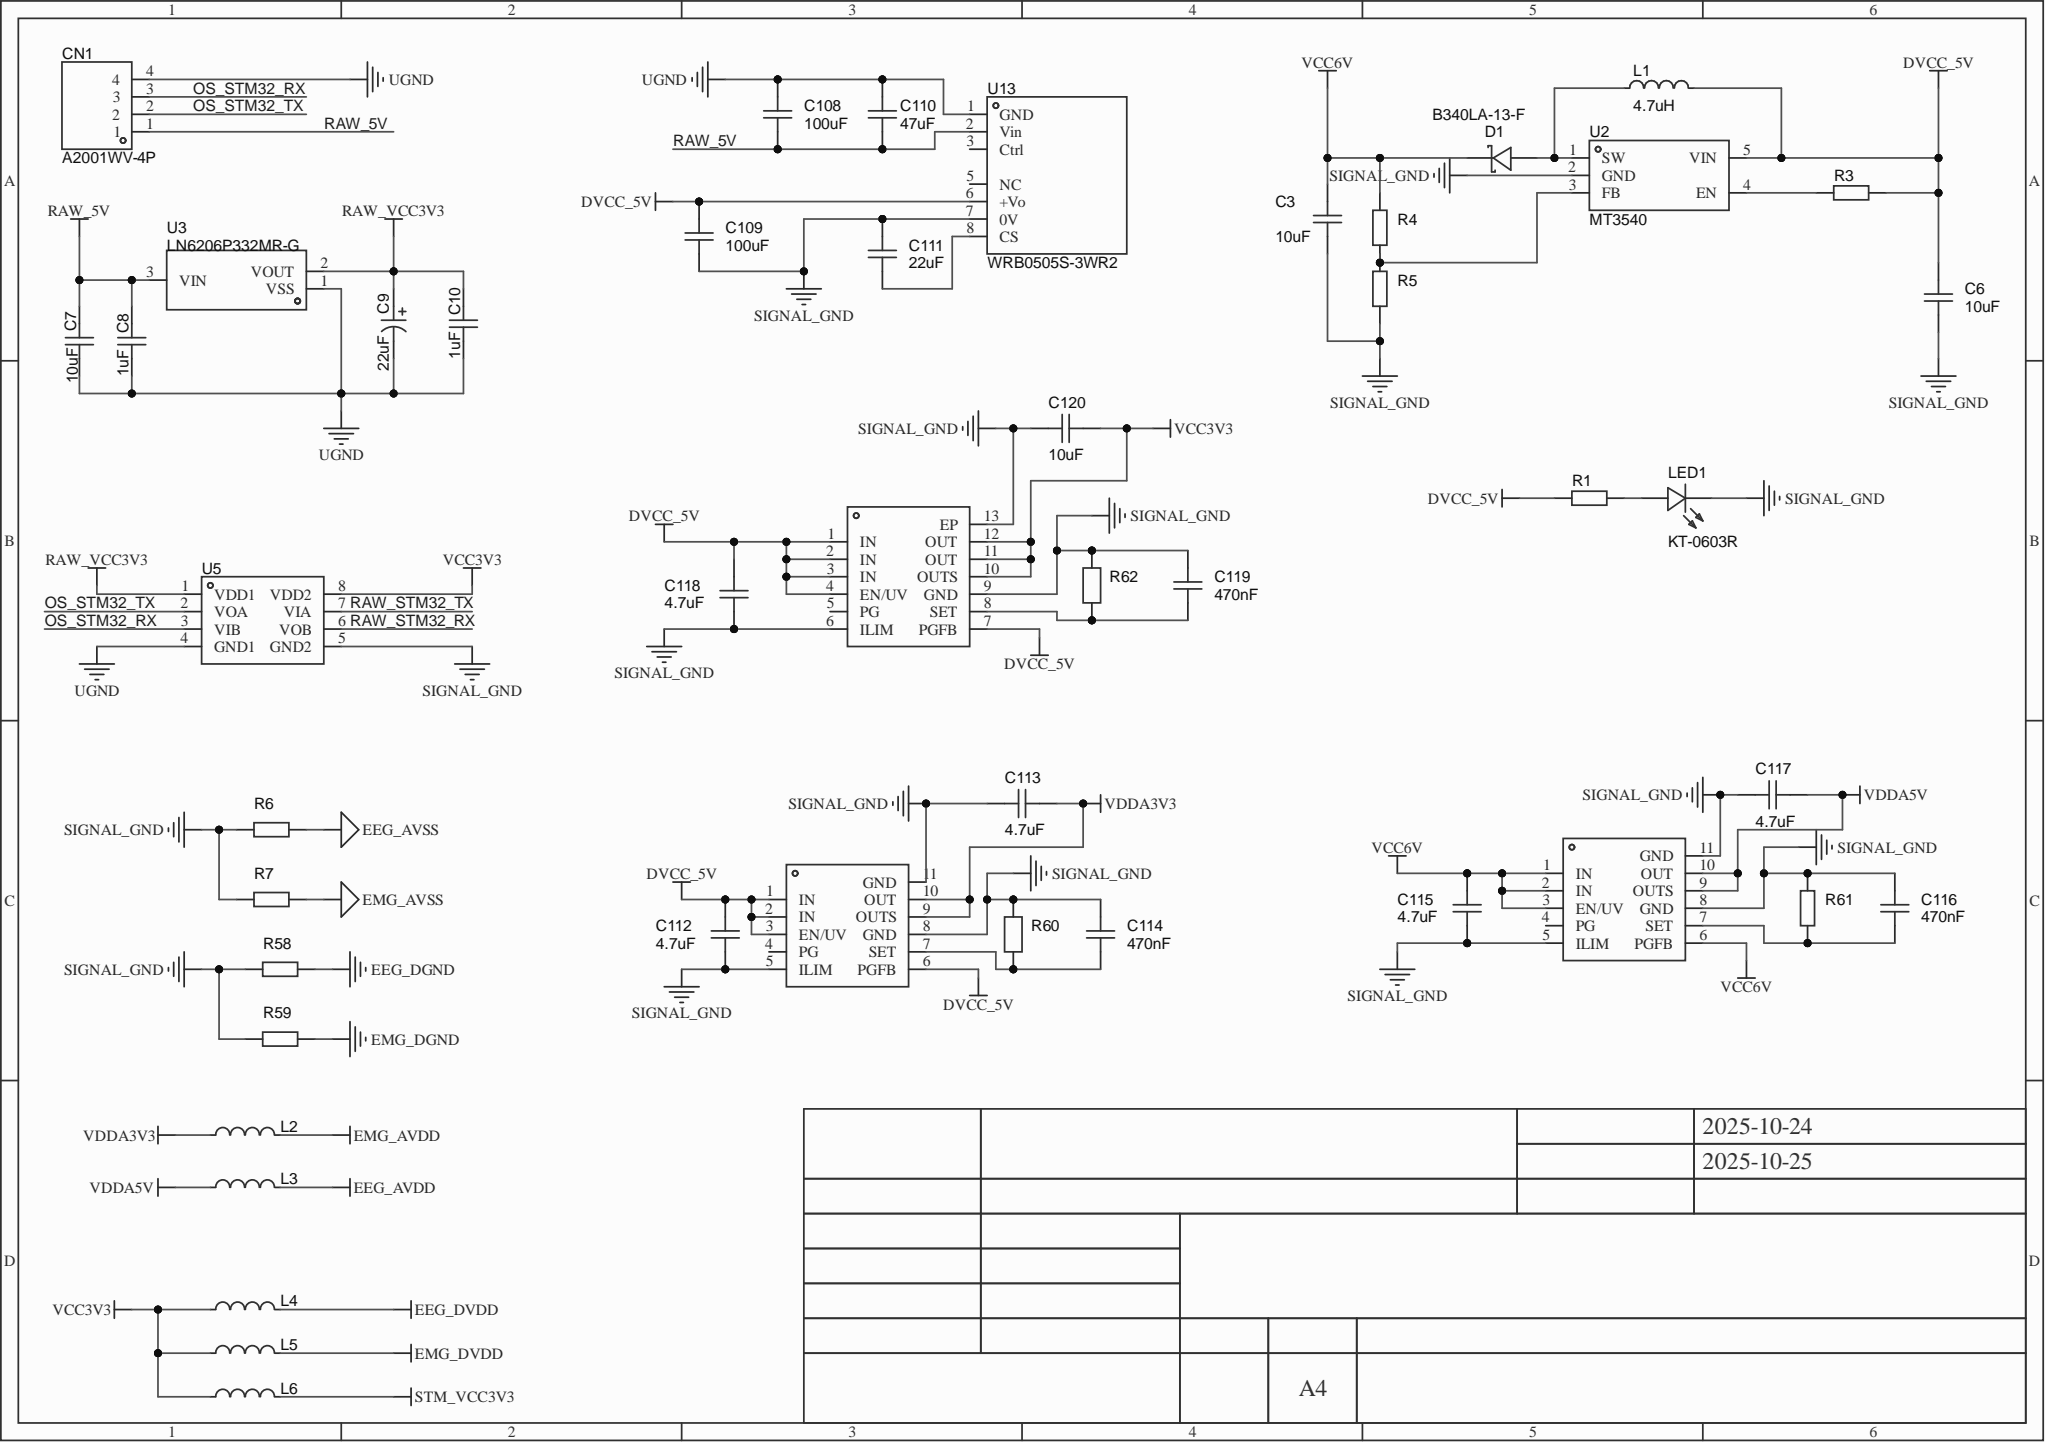Circuit board | Altium Designer | 211 parts | 126 nets | one sheet of the schematic
Parts on this sheet (reference | value | footprint):
C3 | 10uF | C0603
C6 | 10uF | C0603
C7 | 10uF | C0603
C8 | 1uF | C0402
C9 | 22uF | CAP-SMD_L3.2-W1.6
C10 | 1uF | C0402
C108 | 100uF | C1206
C109 | 100uF | C1206
C110 | 47uF | C1206
C111 | 22uF | C1206
C112 | 4.7uF | C0603
C113 | 4.7uF | C0603
C114 | 470nF | C0603
C115 | 4.7uF | C0603
C116 | 470nF | C0603
C117 | 4.7uF | C0603
C118 | 4.7uF | C0603
C119 | 470nF | C0603
C120 | 10uF | C0603
CN1 | A2001WV-4P | CONN-TH_A2001WV-4P
D1 | B340LA-13-F | SMA_L4.3-W2.6-LS5.2-RD
L1 | 4.7uH | IND-SMD_L4.0-W4.0_FNR40XXS
L2 | BLM15PD121SN1D | L0402
L3 | BLM15PD121SN1D | L0402
L4 | BLM15PD121SN1D | L0402
L5 | BLM15PD121SN1D | L0402
L6 | BLM15PD121SN1D | L0402
LED1 | KT-0603R | LED0603-RD
R1 | R0603
R3 | R0402
R4 | R0402
R5 | R0402
R6 | R0402
R7 | R0402
R58 | R0402
R59 | R0402
R60 | R0603
R61 | R0603
R62 | R0603
U2 | MT3540 | SOT-23-5_L3.0-W1.7-P0.95-LS2.8-BR
U3 | LN6206P332MR-G | SOT-23-3_L2.9-W1.3-P1.90-LS2.4-BR
U5 | SOIC-8_L4.9-W3.9-P1.27-LS6.0-BL
U13 | WRB0505S-3WR2 | PWRM-TH_WRA0512S-3WR2
Nets of these parts (net: part-pin ...):
VDDA5V: C117-1 L3-1
VDDA3V3: C113-1 L2-1
VCC6V: C3-2 C115-2 D1-1 R4-2
VCC3V3: C120-2 L4-1 L5-1 L6-1 U5-8
UGND: C7-1 C8-1 C9-2 C10-1 C108-2 C110-2 CN1-4 U3-1 U5-4 U13-1
STM_VCC3V3: L6-2
SIGNAL_GND: C3-1 C6-1 C109-2 C111-2 C112-1 C113-2 C114-1 C115-1 C116-1 C117-2 C118-1 C119-1 C120-1 LED1-1 R5-1 R6-2 R7-2 R58-2 R59-2 R60-1 R61-2 R62-1 U2-2 U5-5 U13-7
RAW_VCC3V3: C9-1 C10-2 U3-2 U5-1
RAW_STM32_TX: U5-7
RAW_STM32_RX: U5-6
RAW_5V: C7-2 C8-2 C108-1 C110-1 CN1-1 U3-3 U13-2
OS_STM32_TX: CN1-2 U5-2
OS_STM32_RX: CN1-3 U5-3
NetR4_1: R4-1 R5-2 U2-3
NetR3_1: R3-1 U2-4
NetLED1_2: LED1-2 R1-2
NetD1_2: D1-2 L1-1 U2-1
NetC119_2: C119-2 R62-2
NetC116_2: C116-2 R61-1
NetC114_2: C114-2 R60-2
NetC111_1: C111-1 U13-8
EMG_DVDD_1: L5-2
EMG_DGND_1: R59-1
EMG_AVSS1: R7-1
EMG_AVDD1: L2-2
EEG_DVDD_1: L4-2
EEG_DGND_1: R58-1
EEG_AVSS1: R6-1
EEG_AVDD1: L3-2
DVCC_5V: C6-2 C109-1 C112-2 C118-2 L1-2 R1-1 R3-2 U2-5 U13-6